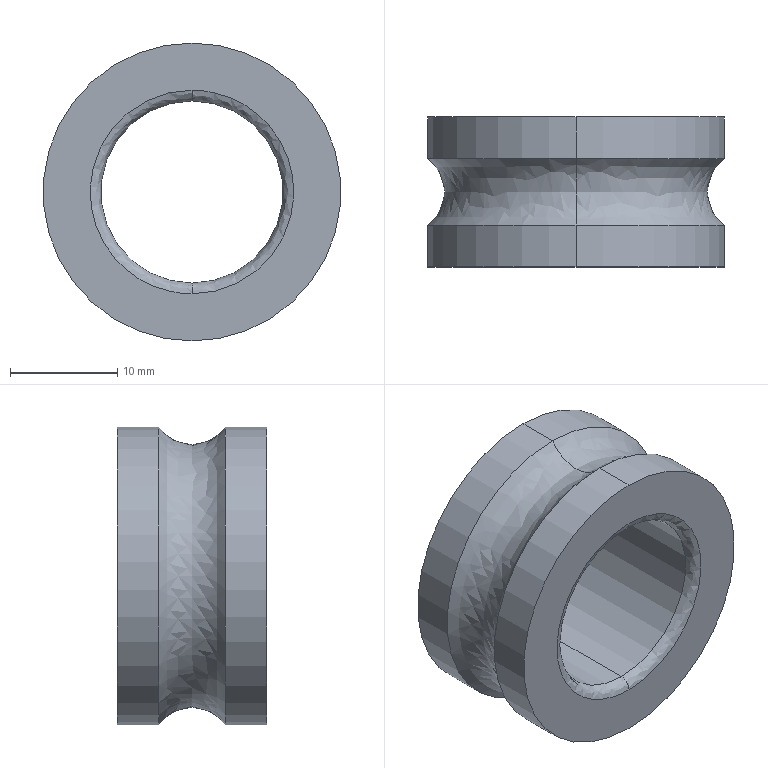Part | SolidWorks | features BaseBody 1 | 1 solid | 14 faces | box 27.8 x 14 x 27.8 mm | volume 4698 mm3 | spline 6 | cylinder 6 | plane 2 | commonest cylinder face diameters 27.8 x4 17 x2
STEP:
#1=CARTESIAN_POINT('',(0.,7.,9.5));
#2=VERTEX_POINT('',#1);
#3=CARTESIAN_POINT('',(0.,7.,-9.5));
#4=VERTEX_POINT('',#3);
#5=CARTESIAN_POINT('',(0.,7.,9.5));
#6=CARTESIAN_POINT('',(19.,7.,9.5));
#7=CARTESIAN_POINT('',(19.,7.,-9.5));
#8=CARTESIAN_POINT('',(0.,7.,-9.5));
#9=(BOUNDED_CURVE()B_SPLINE_CURVE(3,(#5,#6,#7,#8),.UNSPECIFIED.,.F.,.F.)B_SPLINE_CURVE_WITH_KNOTS((4,4),(0.,1.),.UNSPECIFIED.)CURVE()GEOMETRIC_REPRESENTATION_ITEM()RATIONAL_B_SPLINE_CURVE((1.,0.3333,0.3333,1.))REPRESENTATION_ITEM(''));
#10=EDGE_CURVE('',#2,#4,#9,.T.);
#11=ORIENTED_EDGE('',*,*,#10,.T.);
#12=CARTESIAN_POINT('',(0.,6.,-8.5));
#13=VERTEX_POINT('',#12);
#14=CARTESIAN_POINT('',(0.,6.,-9.5));
#15=DIRECTION('',(1.,0.,0.));
#16=DIRECTION('',(0.,0.,-1.));
#17=AXIS2_PLACEMENT_3D('',#14,#15,#16);
#18=CIRCLE('',#17,1.);
#19=EDGE_CURVE('',#4,#13,#18,.T.);
#20=ORIENTED_EDGE('',*,*,#19,.T.);
#21=CARTESIAN_POINT('',(0.,6.,8.5));
#22=VERTEX_POINT('',#21);
#23=CARTESIAN_POINT('',(0.,6.,0.));
#24=DIRECTION('',(0.,-1.,0.));
#25=DIRECTION('',(0.,0.,1.));
#26=AXIS2_PLACEMENT_3D('',#23,#24,#25);
#27=CIRCLE('',#26,8.5);
#28=EDGE_CURVE('',#13,#22,#27,.T.);
#29=ORIENTED_EDGE('',*,*,#28,.T.);
#30=CARTESIAN_POINT('',(0.,6.,9.5));
#31=DIRECTION('',(-1.,0.,0.));
#32=DIRECTION('',(0.,0.,1.));
#33=AXIS2_PLACEMENT_3D('',#30,#31,#32);
#34=CIRCLE('',#33,1.);
#35=EDGE_CURVE('',#2,#22,#34,.T.);
#36=ORIENTED_EDGE('',*,*,#35,.F.);
#37=EDGE_LOOP('',(#11,#20,#29,#36));
#38=FACE_OUTER_BOUND('',#37,.T.);
#39=CARTESIAN_POINT('',(0.,7.,-9.5));
#40=CARTESIAN_POINT('',(19.,7.,-9.5));
#41=CARTESIAN_POINT('',(19.,7.,9.5));
#42=CARTESIAN_POINT('',(0.,7.,9.5));
#43=CARTESIAN_POINT('',(0.,7.,-8.914));
#44=CARTESIAN_POINT('',(17.828,7.,-8.914));
#45=CARTESIAN_POINT('',(17.828,7.,8.914));
#46=CARTESIAN_POINT('',(0.,7.,8.914));
#47=CARTESIAN_POINT('',(0.,6.586,-8.5));
#48=CARTESIAN_POINT('',(17.,6.586,-8.5));
#49=CARTESIAN_POINT('',(17.,6.586,8.5));
#50=CARTESIAN_POINT('',(0.,6.586,8.5));
#51=CARTESIAN_POINT('',(0.,6.,-8.5));
#52=CARTESIAN_POINT('',(17.,6.,-8.5));
#53=CARTESIAN_POINT('',(17.,6.,8.5));
#54=CARTESIAN_POINT('',(0.,6.,8.5));
#55=(BOUNDED_SURFACE()B_SPLINE_SURFACE(3,3,((#39,#40,#41,#42),(#43,#44,#45,#46),(#47,#48,#49,#50),(#51,#52,#53,#54)),.UNSPECIFIED.,.F.,.F.,.F.)B_SPLINE_SURFACE_WITH_KNOTS((4,4),(4,4),(0.,1.),(0.,1.),.UNSPECIFIED.)GEOMETRIC_REPRESENTATION_ITEM()RATIONAL_B_SPLINE_SURFACE(((1.,0.3333,0.3333,1.),(0.8047,0.2682,0.2682,0.8047),(0.8047,0.2682,0.2682,0.8047),(1.,0.3333,0.3333,1.)))REPRESENTATION_ITEM('')SURFACE());
#56=ADVANCED_FACE('',(#38),#55,.T.);
#57=CARTESIAN_POINT('',(0.,3.107,-13.9));
#58=VERTEX_POINT('',#57);
#59=CARTESIAN_POINT('',(0.,3.107,13.9));
#60=VERTEX_POINT('',#59);
#61=CARTESIAN_POINT('',(0.,3.107,0.));
#62=DIRECTION('',(0.,1.,0.));
#63=DIRECTION('',(0.,0.,-1.));
#64=AXIS2_PLACEMENT_3D('',#61,#62,#63);
#65=CIRCLE('',#64,13.9);
#66=EDGE_CURVE('',#58,#60,#65,.T.);
#67=ORIENTED_EDGE('',*,*,#66,.F.);
#68=CARTESIAN_POINT('',(0.,-3.107,-13.9));
#69=VERTEX_POINT('',#68);
#70=CARTESIAN_POINT('',(0.,0.,-16.));
#71=DIRECTION('',(1.,0.,0.));
#72=DIRECTION('',(0.,0.,-1.));
#73=AXIS2_PLACEMENT_3D('',#70,#71,#72);
#74=CIRCLE('',#73,3.75);
#75=EDGE_CURVE('',#58,#69,#74,.T.);
#76=ORIENTED_EDGE('',*,*,#75,.T.);
#77=CARTESIAN_POINT('',(0.,-3.107,13.9));
#78=VERTEX_POINT('',#77);
#79=CARTESIAN_POINT('',(0.,-3.107,0.));
#80=DIRECTION('',(0.,-1.,0.));
#81=DIRECTION('',(0.,0.,1.));
#82=AXIS2_PLACEMENT_3D('',#79,#80,#81);
#83=CIRCLE('',#82,13.9);
#84=EDGE_CURVE('',#78,#69,#83,.T.);
#85=ORIENTED_EDGE('',*,*,#84,.F.);
#86=CARTESIAN_POINT('',(0.,0.,16.));
#87=DIRECTION('',(-1.,0.,0.));
#88=DIRECTION('',(0.,0.,1.));
#89=AXIS2_PLACEMENT_3D('',#86,#87,#88);
#90=CIRCLE('',#89,3.75);
#91=EDGE_CURVE('',#60,#78,#90,.T.);
#92=ORIENTED_EDGE('',*,*,#91,.F.);
#93=EDGE_LOOP('',(#67,#76,#85,#92));
#94=FACE_OUTER_BOUND('',#93,.T.);
#95=CARTESIAN_POINT('',(0.,3.107,13.9));
#96=CARTESIAN_POINT('',(-27.8,3.107,13.9));
#97=CARTESIAN_POINT('',(-27.8,3.107,-13.9));
#98=CARTESIAN_POINT('',(0.,3.107,-13.9));
#99=CARTESIAN_POINT('',(0.,1.465,11.472));
#100=CARTESIAN_POINT('',(-22.943,1.465,11.472));
#101=CARTESIAN_POINT('',(-22.943,1.465,-11.472));
#102=CARTESIAN_POINT('',(0.,1.465,-11.472));
#103=CARTESIAN_POINT('',(0.,-1.465,11.472));
#104=CARTESIAN_POINT('',(-22.943,-1.465,11.472));
#105=CARTESIAN_POINT('',(-22.943,-1.465,-11.472));
#106=CARTESIAN_POINT('',(0.,-1.465,-11.472));
#107=CARTESIAN_POINT('',(0.,-3.107,13.9));
#108=CARTESIAN_POINT('',(-27.8,-3.107,13.9));
#109=CARTESIAN_POINT('',(-27.8,-3.107,-13.9));
#110=CARTESIAN_POINT('',(0.,-3.107,-13.9));
#111=(BOUNDED_SURFACE()B_SPLINE_SURFACE(3,3,((#95,#96,#97,#98),(#99,#100,#101,#102),(#103,#104,#105,#106),(#107,#108,#109,#110)),.UNSPECIFIED.,.F.,.F.,.F.)B_SPLINE_SURFACE_WITH_KNOTS((4,4),(4,4),(0.,1.),(0.,1.),.UNSPECIFIED.)GEOMETRIC_REPRESENTATION_ITEM()RATIONAL_B_SPLINE_SURFACE(((1.,0.3333,0.3333,1.),(0.7067,0.2356,0.2356,0.7067),(0.7067,0.2356,0.2356,0.7067),(1.,0.3333,0.3333,1.)))REPRESENTATION_ITEM('')SURFACE());
#112=ADVANCED_FACE('',(#94),#111,.F.);
#113=CARTESIAN_POINT('',(0.,-6.,8.5));
#114=VERTEX_POINT('',#113);
#115=CARTESIAN_POINT('',(0.,-6.,-8.5));
#116=VERTEX_POINT('',#115);
#117=CARTESIAN_POINT('',(0.,-6.,0.));
#118=DIRECTION('',(0.,1.,0.));
#119=DIRECTION('',(0.,0.,-1.));
#120=AXIS2_PLACEMENT_3D('',#117,#118,#119);
#121=CIRCLE('',#120,8.5);
#122=EDGE_CURVE('',#114,#116,#121,.T.);
#123=ORIENTED_EDGE('',*,*,#122,.T.);
#124=CARTESIAN_POINT('',(0.,-7.,-9.5));
#125=VERTEX_POINT('',#124);
#126=CARTESIAN_POINT('',(0.,-6.,-9.5));
#127=DIRECTION('',(1.,0.,0.));
#128=DIRECTION('',(0.,0.,-1.));
#129=AXIS2_PLACEMENT_3D('',#126,#127,#128);
#130=CIRCLE('',#129,1.);
#131=EDGE_CURVE('',#116,#125,#130,.T.);
#132=ORIENTED_EDGE('',*,*,#131,.T.);
#133=CARTESIAN_POINT('',(0.,-7.,9.5));
#134=VERTEX_POINT('',#133);
#135=CARTESIAN_POINT('',(0.,-7.,-9.5));
#136=CARTESIAN_POINT('',(19.,-7.,-9.5));
#137=CARTESIAN_POINT('',(19.,-7.,9.5));
#138=CARTESIAN_POINT('',(0.,-7.,9.5));
#139=(BOUNDED_CURVE()B_SPLINE_CURVE(3,(#135,#136,#137,#138),.UNSPECIFIED.,.F.,.F.)B_SPLINE_CURVE_WITH_KNOTS((4,4),(0.,1.),.UNSPECIFIED.)CURVE()GEOMETRIC_REPRESENTATION_ITEM()RATIONAL_B_SPLINE_CURVE((1.,0.3333,0.3333,1.))REPRESENTATION_ITEM(''));
#140=EDGE_CURVE('',#125,#134,#139,.T.);
#141=ORIENTED_EDGE('',*,*,#140,.T.);
#142=CARTESIAN_POINT('',(0.,-6.,9.5));
#143=DIRECTION('',(-1.,0.,0.));
#144=DIRECTION('',(0.,0.,1.));
#145=AXIS2_PLACEMENT_3D('',#142,#143,#144);
#146=CIRCLE('',#145,1.);
#147=EDGE_CURVE('',#114,#134,#146,.T.);
#148=ORIENTED_EDGE('',*,*,#147,.F.);
#149=EDGE_LOOP('',(#123,#132,#141,#148));
#150=FACE_OUTER_BOUND('',#149,.T.);
#151=CARTESIAN_POINT('',(0.,-6.,-8.5));
#152=CARTESIAN_POINT('',(17.,-6.,-8.5));
#153=CARTESIAN_POINT('',(17.,-6.,8.5));
#154=CARTESIAN_POINT('',(0.,-6.,8.5));
#155=CARTESIAN_POINT('',(0.,-6.586,-8.5));
#156=CARTESIAN_POINT('',(17.,-6.586,-8.5));
#157=CARTESIAN_POINT('',(17.,-6.586,8.5));
#158=CARTESIAN_POINT('',(0.,-6.586,8.5));
#159=CARTESIAN_POINT('',(0.,-7.,-8.914));
#160=CARTESIAN_POINT('',(17.828,-7.,-8.914));
#161=CARTESIAN_POINT('',(17.828,-7.,8.914));
#162=CARTESIAN_POINT('',(0.,-7.,8.914));
#163=CARTESIAN_POINT('',(0.,-7.,-9.5));
#164=CARTESIAN_POINT('',(19.,-7.,-9.5));
#165=CARTESIAN_POINT('',(19.,-7.,9.5));
#166=CARTESIAN_POINT('',(0.,-7.,9.5));
#167=(BOUNDED_SURFACE()B_SPLINE_SURFACE(3,3,((#151,#152,#153,#154),(#155,#156,#157,#158),(#159,#160,#161,#162),(#163,#164,#165,#166)),.UNSPECIFIED.,.F.,.F.,.T.)B_SPLINE_SURFACE_WITH_KNOTS((4,4),(4,4),(0.,1.),(0.,1.),.UNSPECIFIED.)GEOMETRIC_REPRESENTATION_ITEM()RATIONAL_B_SPLINE_SURFACE(((1.,0.3333,0.3333,1.),(0.8047,0.2682,0.2682,0.8047),(0.8047,0.2682,0.2682,0.8047),(1.,0.3333,0.3333,1.)))REPRESENTATION_ITEM('')SURFACE());
#168=ADVANCED_FACE('',(#150),#167,.T.);
#169=CARTESIAN_POINT('',(0.,7.,-13.9));
#170=VERTEX_POINT('',#169);
#171=CARTESIAN_POINT('',(0.,7.,13.9));
#172=VERTEX_POINT('',#171);
#173=CARTESIAN_POINT('',(0.,7.,0.));
#174=DIRECTION('',(0.,-1.,0.));
#175=DIRECTION('',(0.,0.,-1.));
#176=AXIS2_PLACEMENT_3D('',#173,#174,#175);
#177=CIRCLE('',#176,13.9);
#178=EDGE_CURVE('',#170,#172,#177,.T.);
#179=ORIENTED_EDGE('',*,*,#178,.T.);
#180=CARTESIAN_POINT('',(0.,7.7,13.9));
#181=DIRECTION('',(0.,-1.,0.));
#182=VECTOR('',#181,1000.);
#183=LINE('',#180,#182);
#184=EDGE_CURVE('',#172,#60,#183,.T.);
#185=ORIENTED_EDGE('',*,*,#184,.T.);
#186=CARTESIAN_POINT('',(0.,3.107,0.));
#187=DIRECTION('',(0.,1.,0.));
#188=DIRECTION('',(0.,0.,-1.));
#189=AXIS2_PLACEMENT_3D('',#186,#187,#188);
#190=CIRCLE('',#189,13.9);
#191=EDGE_CURVE('',#60,#58,#190,.T.);
#192=ORIENTED_EDGE('',*,*,#191,.T.);
#193=CARTESIAN_POINT('',(0.,7.7,-13.9));
#194=DIRECTION('',(0.,-1.,0.));
#195=VECTOR('',#194,1000.);
#196=LINE('',#193,#195);
#197=EDGE_CURVE('',#170,#58,#196,.T.);
#198=ORIENTED_EDGE('',*,*,#197,.F.);
#199=EDGE_LOOP('',(#179,#185,#192,#198));
#200=FACE_OUTER_BOUND('',#199,.T.);
#201=CARTESIAN_POINT('',(0.,7.7,0.));
#202=DIRECTION('',(0.,-1.,0.));
#203=DIRECTION('',(0.,0.,-1.));
#204=AXIS2_PLACEMENT_3D('',#201,#202,#203);
#205=CYLINDRICAL_SURFACE('',#204,13.9);
#206=ADVANCED_FACE('',(#200),#205,.T.);
#207=CARTESIAN_POINT('',(0.,6.,0.));
#208=DIRECTION('',(0.,-1.,0.));
#209=DIRECTION('',(0.,0.,1.));
#210=AXIS2_PLACEMENT_3D('',#207,#208,#209);
#211=CIRCLE('',#210,8.5);
#212=EDGE_CURVE('',#22,#13,#211,.T.);
#213=ORIENTED_EDGE('',*,*,#212,.F.);
#214=CARTESIAN_POINT('',(0.,7.7,8.5));
#215=DIRECTION('',(0.,-1.,0.));
#216=VECTOR('',#215,1000.);
#217=LINE('',#214,#216);
#218=EDGE_CURVE('',#22,#114,#217,.T.);
#219=ORIENTED_EDGE('',*,*,#218,.T.);
#220=CARTESIAN_POINT('',(0.,-6.,0.));
#221=DIRECTION('',(0.,1.,0.));
#222=DIRECTION('',(0.,0.,-1.));
#223=AXIS2_PLACEMENT_3D('',#220,#221,#222);
#224=CIRCLE('',#223,8.5);
#225=EDGE_CURVE('',#116,#114,#224,.T.);
#226=ORIENTED_EDGE('',*,*,#225,.F.);
#227=CARTESIAN_POINT('',(0.,7.7,-8.5));
#228=DIRECTION('',(0.,-1.,0.));
#229=VECTOR('',#228,1000.);
#230=LINE('',#227,#229);
#231=EDGE_CURVE('',#13,#116,#230,.T.);
#232=ORIENTED_EDGE('',*,*,#231,.F.);
#233=EDGE_LOOP('',(#213,#219,#226,#232));
#234=FACE_OUTER_BOUND('',#233,.T.);
#235=CARTESIAN_POINT('',(0.,7.7,0.));
#236=DIRECTION('',(0.,-1.,0.));
#237=DIRECTION('',(0.,0.,-1.));
#238=AXIS2_PLACEMENT_3D('',#235,#236,#237);
#239=CYLINDRICAL_SURFACE('',#238,8.5);
#240=ADVANCED_FACE('',(#234),#239,.F.);
#241=CARTESIAN_POINT('',(0.,-3.107,0.));
#242=DIRECTION('',(0.,-1.,0.));
#243=DIRECTION('',(0.,0.,1.));
#244=AXIS2_PLACEMENT_3D('',#241,#242,#243);
#245=CIRCLE('',#244,13.9);
#246=EDGE_CURVE('',#69,#78,#245,.T.);
#247=ORIENTED_EDGE('',*,*,#246,.T.);
#248=CARTESIAN_POINT('',(0.,-7.,13.9));
#249=VERTEX_POINT('',#248);
#250=CARTESIAN_POINT('',(0.,7.7,13.9));
#251=DIRECTION('',(0.,-1.,0.));
#252=VECTOR('',#251,1000.);
#253=LINE('',#250,#252);
#254=EDGE_CURVE('',#78,#249,#253,.T.);
#255=ORIENTED_EDGE('',*,*,#254,.T.);
#256=CARTESIAN_POINT('',(0.,-7.,-13.9));
#257=VERTEX_POINT('',#256);
#258=CARTESIAN_POINT('',(0.,-7.,0.));
#259=DIRECTION('',(0.,1.,0.));
#260=DIRECTION('',(0.,0.,-1.));
#261=AXIS2_PLACEMENT_3D('',#258,#259,#260);
#262=CIRCLE('',#261,13.9);
#263=EDGE_CURVE('',#249,#257,#262,.T.);
#264=ORIENTED_EDGE('',*,*,#263,.T.);
#265=CARTESIAN_POINT('',(0.,7.7,-13.9));
#266=DIRECTION('',(0.,-1.,0.));
#267=VECTOR('',#266,1000.);
#268=LINE('',#265,#267);
#269=EDGE_CURVE('',#69,#257,#268,.T.);
#270=ORIENTED_EDGE('',*,*,#269,.F.);
#271=EDGE_LOOP('',(#247,#255,#264,#270));
#272=FACE_OUTER_BOUND('',#271,.T.);
#273=CARTESIAN_POINT('',(0.,7.7,0.));
#274=DIRECTION('',(0.,-1.,0.));
#275=DIRECTION('',(0.,0.,-1.));
#276=AXIS2_PLACEMENT_3D('',#273,#274,#275);
#277=CYLINDRICAL_SURFACE('',#276,13.9);
#278=ADVANCED_FACE('',(#272),#277,.T.);
#279=ORIENTED_EDGE('',*,*,#10,.F.);
#280=CARTESIAN_POINT('',(0.,7.,-9.5));
#281=CARTESIAN_POINT('',(-19.,7.,-9.5));
#282=CARTESIAN_POINT('',(-19.,7.,9.5));
#283=CARTESIAN_POINT('',(0.,7.,9.5));
#284=(BOUNDED_CURVE()B_SPLINE_CURVE(3,(#280,#281,#282,#283),.UNSPECIFIED.,.F.,.F.)B_SPLINE_CURVE_WITH_KNOTS((4,4),(0.,1.),.UNSPECIFIED.)CURVE()GEOMETRIC_REPRESENTATION_ITEM()RATIONAL_B_SPLINE_CURVE((1.,0.3333,0.3333,1.))REPRESENTATION_ITEM(''));
#285=EDGE_CURVE('',#4,#2,#284,.T.);
#286=ORIENTED_EDGE('',*,*,#285,.F.);
#287=EDGE_LOOP('',(#279,#286));
#288=FACE_BOUND('',#287,.T.);
#289=ORIENTED_EDGE('',*,*,#178,.F.);
#290=CARTESIAN_POINT('',(0.,7.,0.));
#291=DIRECTION('',(0.,-1.,0.));
#292=DIRECTION('',(0.,0.,-1.));
#293=AXIS2_PLACEMENT_3D('',#290,#291,#292);
#294=CIRCLE('',#293,13.9);
#295=EDGE_CURVE('',#172,#170,#294,.T.);
#296=ORIENTED_EDGE('',*,*,#295,.F.);
#297=EDGE_LOOP('',(#289,#296));
#298=FACE_OUTER_BOUND('',#297,.T.);
#299=CARTESIAN_POINT('',(0.,7.,0.));
#300=DIRECTION('',(0.,-1.,0.));
#301=DIRECTION('',(0.,0.,-1.));
#302=AXIS2_PLACEMENT_3D('',#299,#300,#301);
#303=PLANE('',#302);
#304=ADVANCED_FACE('',(#288,#298),#303,.F.);
#305=ORIENTED_EDGE('',*,*,#19,.F.);
#306=ORIENTED_EDGE('',*,*,#285,.T.);
#307=ORIENTED_EDGE('',*,*,#35,.T.);
#308=ORIENTED_EDGE('',*,*,#212,.T.);
#309=EDGE_LOOP('',(#305,#306,#307,#308));
#310=FACE_OUTER_BOUND('',#309,.T.);
#311=CARTESIAN_POINT('',(0.,7.,9.5));
#312=CARTESIAN_POINT('',(-19.,7.,9.5));
#313=CARTESIAN_POINT('',(-19.,7.,-9.5));
#314=CARTESIAN_POINT('',(0.,7.,-9.5));
#315=CARTESIAN_POINT('',(0.,7.,8.914));
#316=CARTESIAN_POINT('',(-17.828,7.,8.914));
#317=CARTESIAN_POINT('',(-17.828,7.,-8.914));
#318=CARTESIAN_POINT('',(0.,7.,-8.914));
#319=CARTESIAN_POINT('',(0.,6.586,8.5));
#320=CARTESIAN_POINT('',(-17.,6.586,8.5));
#321=CARTESIAN_POINT('',(-17.,6.586,-8.5));
#322=CARTESIAN_POINT('',(0.,6.586,-8.5));
#323=CARTESIAN_POINT('',(0.,6.,8.5));
#324=CARTESIAN_POINT('',(-17.,6.,8.5));
#325=CARTESIAN_POINT('',(-17.,6.,-8.5));
#326=CARTESIAN_POINT('',(0.,6.,-8.5));
#327=(BOUNDED_SURFACE()B_SPLINE_SURFACE(3,3,((#311,#312,#313,#314),(#315,#316,#317,#318),(#319,#320,#321,#322),(#323,#324,#325,#326)),.UNSPECIFIED.,.F.,.F.,.F.)B_SPLINE_SURFACE_WITH_KNOTS((4,4),(4,4),(0.,1.),(0.,1.),.UNSPECIFIED.)GEOMETRIC_REPRESENTATION_ITEM()RATIONAL_B_SPLINE_SURFACE(((1.,0.3333,0.3333,1.),(0.8047,0.2682,0.2682,0.8047),(0.8047,0.2682,0.2682,0.8047),(1.,0.3333,0.3333,1.)))REPRESENTATION_ITEM('')SURFACE());
#328=ADVANCED_FACE('',(#310),#327,.T.);
#329=ORIENTED_EDGE('',*,*,#184,.F.);
#330=ORIENTED_EDGE('',*,*,#295,.T.);
#331=ORIENTED_EDGE('',*,*,#197,.T.);
#332=ORIENTED_EDGE('',*,*,#66,.T.);
#333=EDGE_LOOP('',(#329,#330,#331,#332));
#334=FACE_OUTER_BOUND('',#333,.T.);
#335=CARTESIAN_POINT('',(0.,7.7,0.));
#336=DIRECTION('',(0.,-1.,0.));
#337=DIRECTION('',(0.,0.,-1.));
#338=AXIS2_PLACEMENT_3D('',#335,#336,#337);
#339=CYLINDRICAL_SURFACE('',#338,13.9);
#340=ADVANCED_FACE('',(#334),#339,.T.);
#341=ORIENTED_EDGE('',*,*,#218,.F.);
#342=ORIENTED_EDGE('',*,*,#28,.F.);
#343=ORIENTED_EDGE('',*,*,#231,.T.);
#344=ORIENTED_EDGE('',*,*,#122,.F.);
#345=EDGE_LOOP('',(#341,#342,#343,#344));
#346=FACE_OUTER_BOUND('',#345,.T.);
#347=CARTESIAN_POINT('',(0.,7.7,0.));
#348=DIRECTION('',(0.,-1.,0.));
#349=DIRECTION('',(0.,0.,-1.));
#350=AXIS2_PLACEMENT_3D('',#347,#348,#349);
#351=CYLINDRICAL_SURFACE('',#350,8.5);
#352=ADVANCED_FACE('',(#346),#351,.F.);
#353=ORIENTED_EDGE('',*,*,#75,.F.);
#354=ORIENTED_EDGE('',*,*,#191,.F.);
#355=ORIENTED_EDGE('',*,*,#91,.T.);
#356=ORIENTED_EDGE('',*,*,#246,.F.);
#357=EDGE_LOOP('',(#353,#354,#355,#356));
#358=FACE_OUTER_BOUND('',#357,.T.);
#359=CARTESIAN_POINT('',(0.,3.107,-13.9));
#360=CARTESIAN_POINT('',(27.8,3.107,-13.9));
#361=CARTESIAN_POINT('',(27.8,3.107,13.9));
#362=CARTESIAN_POINT('',(0.,3.107,13.9));
#363=CARTESIAN_POINT('',(0.,1.465,-11.472));
#364=CARTESIAN_POINT('',(22.943,1.465,-11.472));
#365=CARTESIAN_POINT('',(22.943,1.465,11.472));
#366=CARTESIAN_POINT('',(0.,1.465,11.472));
#367=CARTESIAN_POINT('',(0.,-1.465,-11.472));
#368=CARTESIAN_POINT('',(22.943,-1.465,-11.472));
#369=CARTESIAN_POINT('',(22.943,-1.465,11.472));
#370=CARTESIAN_POINT('',(0.,-1.465,11.472));
#371=CARTESIAN_POINT('',(0.,-3.107,-13.9));
#372=CARTESIAN_POINT('',(27.8,-3.107,-13.9));
#373=CARTESIAN_POINT('',(27.8,-3.107,13.9));
#374=CARTESIAN_POINT('',(0.,-3.107,13.9));
#375=(BOUNDED_SURFACE()B_SPLINE_SURFACE(3,3,((#359,#360,#361,#362),(#363,#364,#365,#366),(#367,#368,#369,#370),(#371,#372,#373,#374)),.UNSPECIFIED.,.F.,.F.,.T.)B_SPLINE_SURFACE_WITH_KNOTS((4,4),(4,4),(0.,1.),(0.,1.),.UNSPECIFIED.)GEOMETRIC_REPRESENTATION_ITEM()RATIONAL_B_SPLINE_SURFACE(((1.,0.3333,0.3333,1.),(0.7067,0.2356,0.2356,0.7067),(0.7067,0.2356,0.2356,0.7067),(1.,0.3333,0.3333,1.)))REPRESENTATION_ITEM('')SURFACE());
#376=ADVANCED_FACE('',(#358),#375,.F.);
#377=ORIENTED_EDGE('',*,*,#131,.F.);
#378=ORIENTED_EDGE('',*,*,#225,.T.);
#379=ORIENTED_EDGE('',*,*,#147,.T.);
#380=CARTESIAN_POINT('',(0.,-7.,9.5));
#381=CARTESIAN_POINT('',(-19.,-7.,9.5));
#382=CARTESIAN_POINT('',(-19.,-7.,-9.5));
#383=CARTESIAN_POINT('',(0.,-7.,-9.5));
#384=(BOUNDED_CURVE()B_SPLINE_CURVE(3,(#380,#381,#382,#383),.UNSPECIFIED.,.F.,.F.)B_SPLINE_CURVE_WITH_KNOTS((4,4),(0.,1.),.UNSPECIFIED.)CURVE()GEOMETRIC_REPRESENTATION_ITEM()RATIONAL_B_SPLINE_CURVE((1.,0.3333,0.3333,1.))REPRESENTATION_ITEM(''));
#385=EDGE_CURVE('',#134,#125,#384,.T.);
#386=ORIENTED_EDGE('',*,*,#385,.T.);
#387=EDGE_LOOP('',(#377,#378,#379,#386));
#388=FACE_OUTER_BOUND('',#387,.T.);
#389=CARTESIAN_POINT('',(0.,-6.,8.5));
#390=CARTESIAN_POINT('',(-17.,-6.,8.5));
#391=CARTESIAN_POINT('',(-17.,-6.,-8.5));
#392=CARTESIAN_POINT('',(0.,-6.,-8.5));
#393=CARTESIAN_POINT('',(0.,-6.586,8.5));
#394=CARTESIAN_POINT('',(-17.,-6.586,8.5));
#395=CARTESIAN_POINT('',(-17.,-6.586,-8.5));
#396=CARTESIAN_POINT('',(0.,-6.586,-8.5));
#397=CARTESIAN_POINT('',(0.,-7.,8.914));
#398=CARTESIAN_POINT('',(-17.828,-7.,8.914));
#399=CARTESIAN_POINT('',(-17.828,-7.,-8.914));
#400=CARTESIAN_POINT('',(0.,-7.,-8.914));
#401=CARTESIAN_POINT('',(0.,-7.,9.5));
#402=CARTESIAN_POINT('',(-19.,-7.,9.5));
#403=CARTESIAN_POINT('',(-19.,-7.,-9.5));
#404=CARTESIAN_POINT('',(0.,-7.,-9.5));
#405=(BOUNDED_SURFACE()B_SPLINE_SURFACE(3,3,((#389,#390,#391,#392),(#393,#394,#395,#396),(#397,#398,#399,#400),(#401,#402,#403,#404)),.UNSPECIFIED.,.F.,.F.,.T.)B_SPLINE_SURFACE_WITH_KNOTS((4,4),(4,4),(0.,1.),(0.,1.),.UNSPECIFIED.)GEOMETRIC_REPRESENTATION_ITEM()RATIONAL_B_SPLINE_SURFACE(((1.,0.3333,0.3333,1.),(0.8047,0.2682,0.2682,0.8047),(0.8047,0.2682,0.2682,0.8047),(1.,0.3333,0.3333,1.)))REPRESENTATION_ITEM('')SURFACE());
#406=ADVANCED_FACE('',(#388),#405,.T.);
#407=ORIENTED_EDGE('',*,*,#254,.F.);
#408=ORIENTED_EDGE('',*,*,#84,.T.);
#409=ORIENTED_EDGE('',*,*,#269,.T.);
#410=CARTESIAN_POINT('',(0.,-7.,0.));
#411=DIRECTION('',(0.,1.,0.));
#412=DIRECTION('',(0.,0.,-1.));
#413=AXIS2_PLACEMENT_3D('',#410,#411,#412);
#414=CIRCLE('',#413,13.9);
#415=EDGE_CURVE('',#257,#249,#414,.T.);
#416=ORIENTED_EDGE('',*,*,#415,.T.);
#417=EDGE_LOOP('',(#407,#408,#409,#416));
#418=FACE_OUTER_BOUND('',#417,.T.);
#419=CARTESIAN_POINT('',(0.,7.7,0.));
#420=DIRECTION('',(0.,-1.,0.));
#421=DIRECTION('',(0.,0.,-1.));
#422=AXIS2_PLACEMENT_3D('',#419,#420,#421);
#423=CYLINDRICAL_SURFACE('',#422,13.9);
#424=ADVANCED_FACE('',(#418),#423,.T.);
#425=ORIENTED_EDGE('',*,*,#140,.F.);
#426=ORIENTED_EDGE('',*,*,#385,.F.);
#427=EDGE_LOOP('',(#425,#426));
#428=FACE_BOUND('',#427,.T.);
#429=ORIENTED_EDGE('',*,*,#415,.F.);
#430=ORIENTED_EDGE('',*,*,#263,.F.);
#431=EDGE_LOOP('',(#429,#430));
#432=FACE_OUTER_BOUND('',#431,.T.);
#433=CARTESIAN_POINT('',(0.,-7.,0.));
#434=DIRECTION('',(0.,-1.,0.));
#435=DIRECTION('',(0.,0.,-1.));
#436=AXIS2_PLACEMENT_3D('',#433,#434,#435);
#437=PLANE('',#436);
#438=ADVANCED_FACE('',(#428,#432),#437,.T.);
#439=CLOSED_SHELL('',(#56,#112,#168,#206,#240,#278,#304,#328,#340,#352,#376,#406,#424,#438));
#440=MANIFOLD_SOLID_BREP('',#439);
#441=CARTESIAN_POINT('',(0.,0.,0.));
#442=DIRECTION('',(0.,0.,1.));
#443=DIRECTION('',(1.,0.,0.));
#444=AXIS2_PLACEMENT_3D('',#441,#442,#443);
#445=(LENGTH_UNIT()NAMED_UNIT(*)SI_UNIT(.MILLI.,.METRE.));
#446=UNCERTAINTY_MEASURE_WITH_UNIT(LENGTH_MEASURE(0.00001),#445,'','');
#447=(NAMED_UNIT(*)PLANE_ANGLE_UNIT()SI_UNIT($,.RADIAN.));
#448=(NAMED_UNIT(*)SI_UNIT($,.STERADIAN.)SOLID_ANGLE_UNIT());
#449=(GEOMETRIC_REPRESENTATION_CONTEXT(3)GLOBAL_UNCERTAINTY_ASSIGNED_CONTEXT((#446))GLOBAL_UNIT_ASSIGNED_CONTEXT((#445,#447,#448))REPRESENTATION_CONTEXT('',''));
#450=ADVANCED_BREP_SHAPE_REPRESENTATION('',(#440,#444),#449);